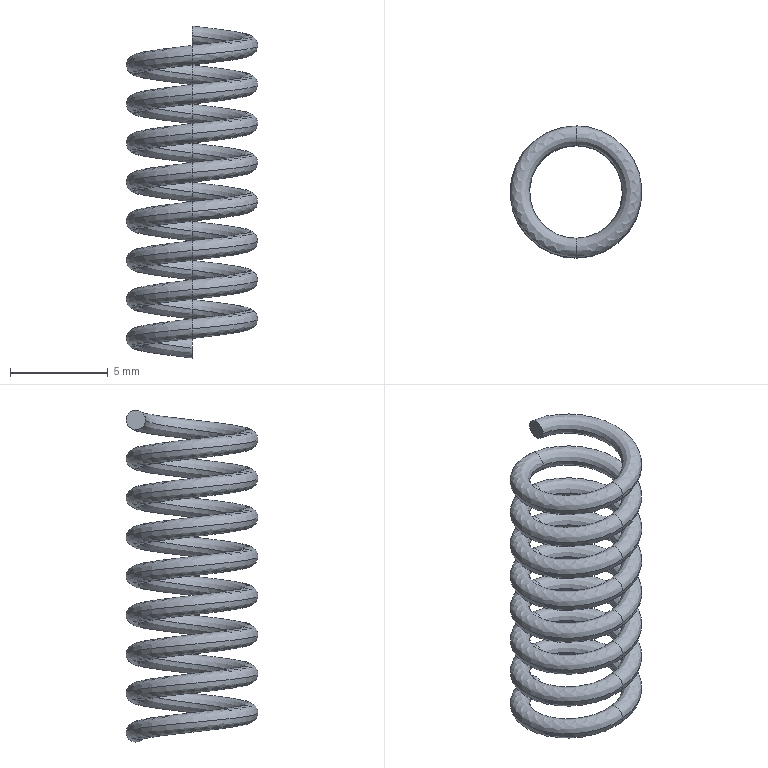Part | CATIA | 1 solid | 34 faces | box 6.75 x 6.75 x 17 mm | volume 113.5 mm3 | spline 32 | plane 2